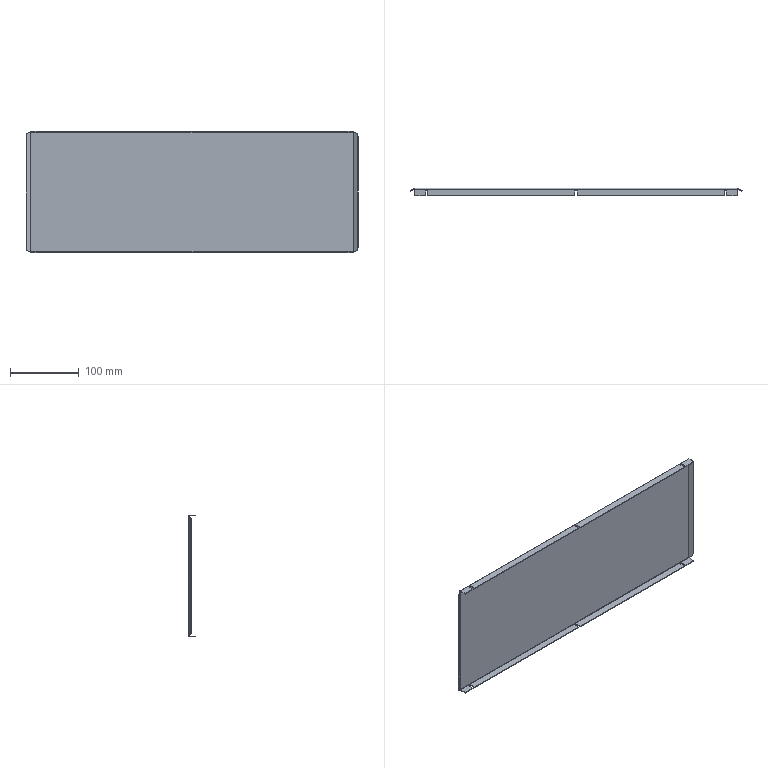Part | SolidWorks | features SplitBody 1 | 1 solid | 70 faces | box 482.174 x 11.2 x 177.1 mm | volume 99218 mm3 | plane 52 | cylinder 18 | commonest cylinder face diameters 3.15 x6 1.031 x4 3.131 x4 14 x4